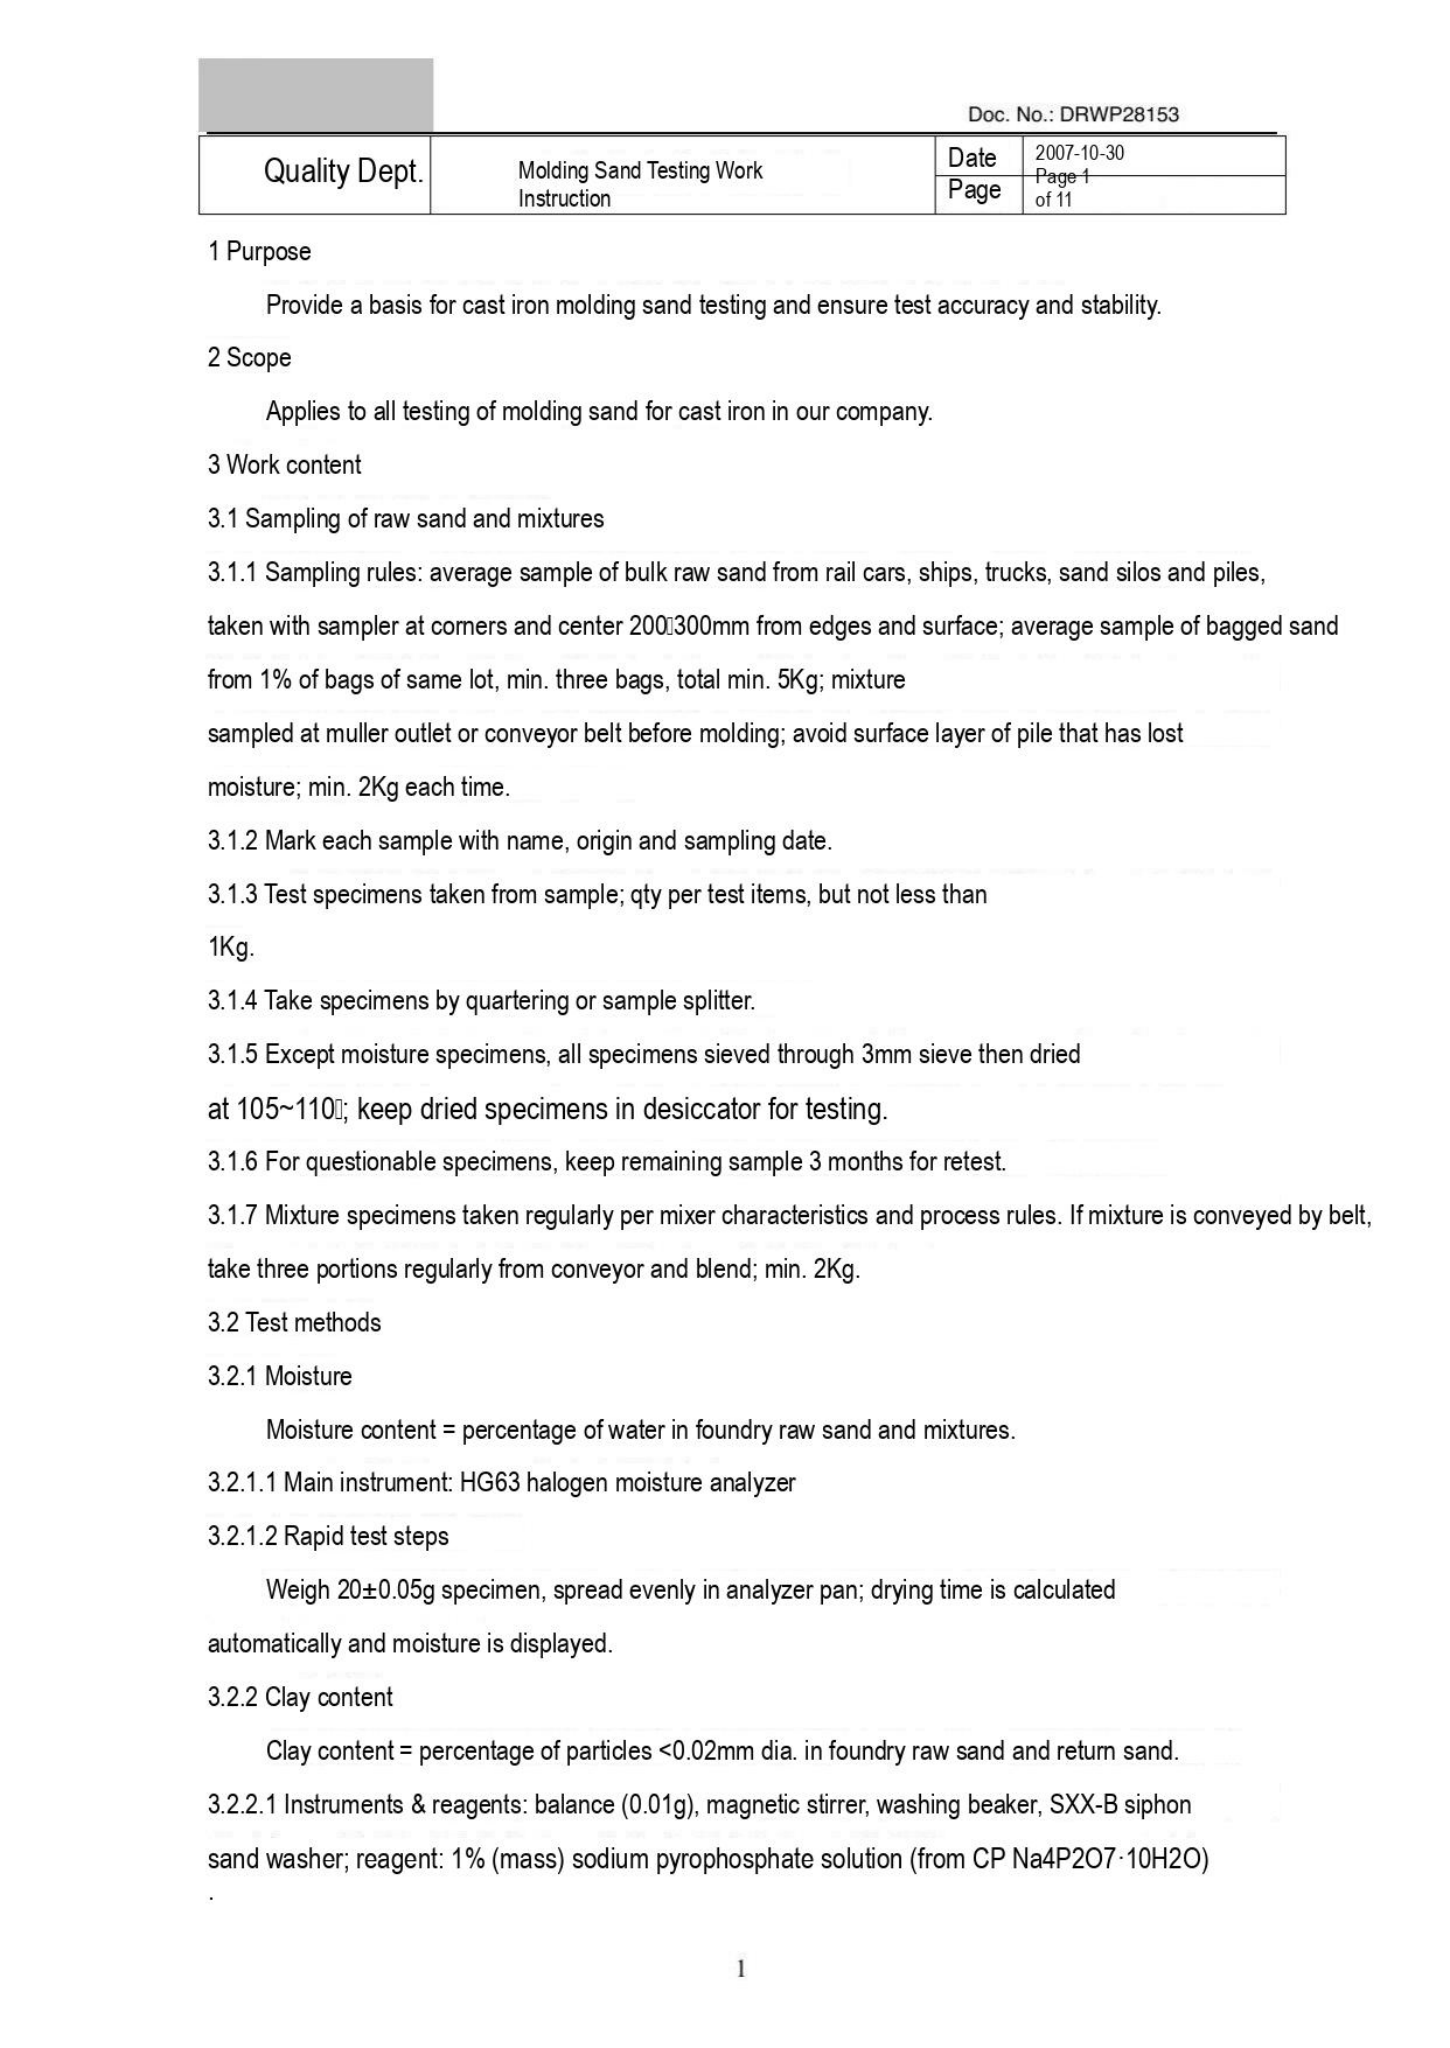Doc. No.: DRWP28153

| Quality Dept. | Molding Sand Testing Work Instruction | Date | 2007-10-30 |
|---|---|---|---|
| | | Page | Page 1 of 11 |

1 Purpose

Provide a basis for cast iron molding sand testing and ensure test accuracy and stability.

2 Scope

Applies to all testing of molding sand for cast iron in our company.

3 Work content

3.1 Sampling of raw sand and mixtures

3.1.1 Sampling rules: average sample of bulk raw sand from rail cars, ships, trucks, sand silos and piles, taken with sampler at corners and center 200300mm from edges and surface; average sample of bagged sand from 1% of bags of same lot, min. three bags, total min. 5Kg; mixture sampled at muller outlet or conveyor belt before molding; avoid surface layer of pile that has lost moisture; min. 2Kg each time.

3.1.2 Mark each sample with name, origin and sampling date.

3.1.3 Test specimens taken from sample; qty per test items, but not less than 1Kg.

3.1.4 Take specimens by quartering or sample splitter.

3.1.5 Except moisture specimens, all specimens sieved through 3mm sieve then dried at 105~110; keep dried specimens in desiccator for testing.

3.1.6 For questionable specimens, keep remaining sample 3 months for retest.

3.1.7 Mixture specimens taken regularly per mixer characteristics and process rules. If mixture is conveyed by belt, take three portions regularly from conveyor and blend; min. 2Kg.

3.2 Test methods

3.2.1 Moisture

Moisture content = percentage of water in foundry raw sand and mixtures.

3.2.1.1 Main instrument: HG63 halogen moisture analyzer

3.2.1.2 Rapid test steps

Weigh 20±0.05g specimen, spread evenly in analyzer pan; drying time is calculated automatically and moisture is displayed.

3.2.2 Clay content

Clay content = percentage of particles <0.02mm dia. in foundry raw sand and return sand.

3.2.2.1 Instruments & reagents: balance (0.01g), magnetic stirrer, washing beaker, SXX-B siphon sand washer; reagent: 1% (mass) sodium pyrophosphate solution (from CP Na4P2O7·10H2O)

.

1
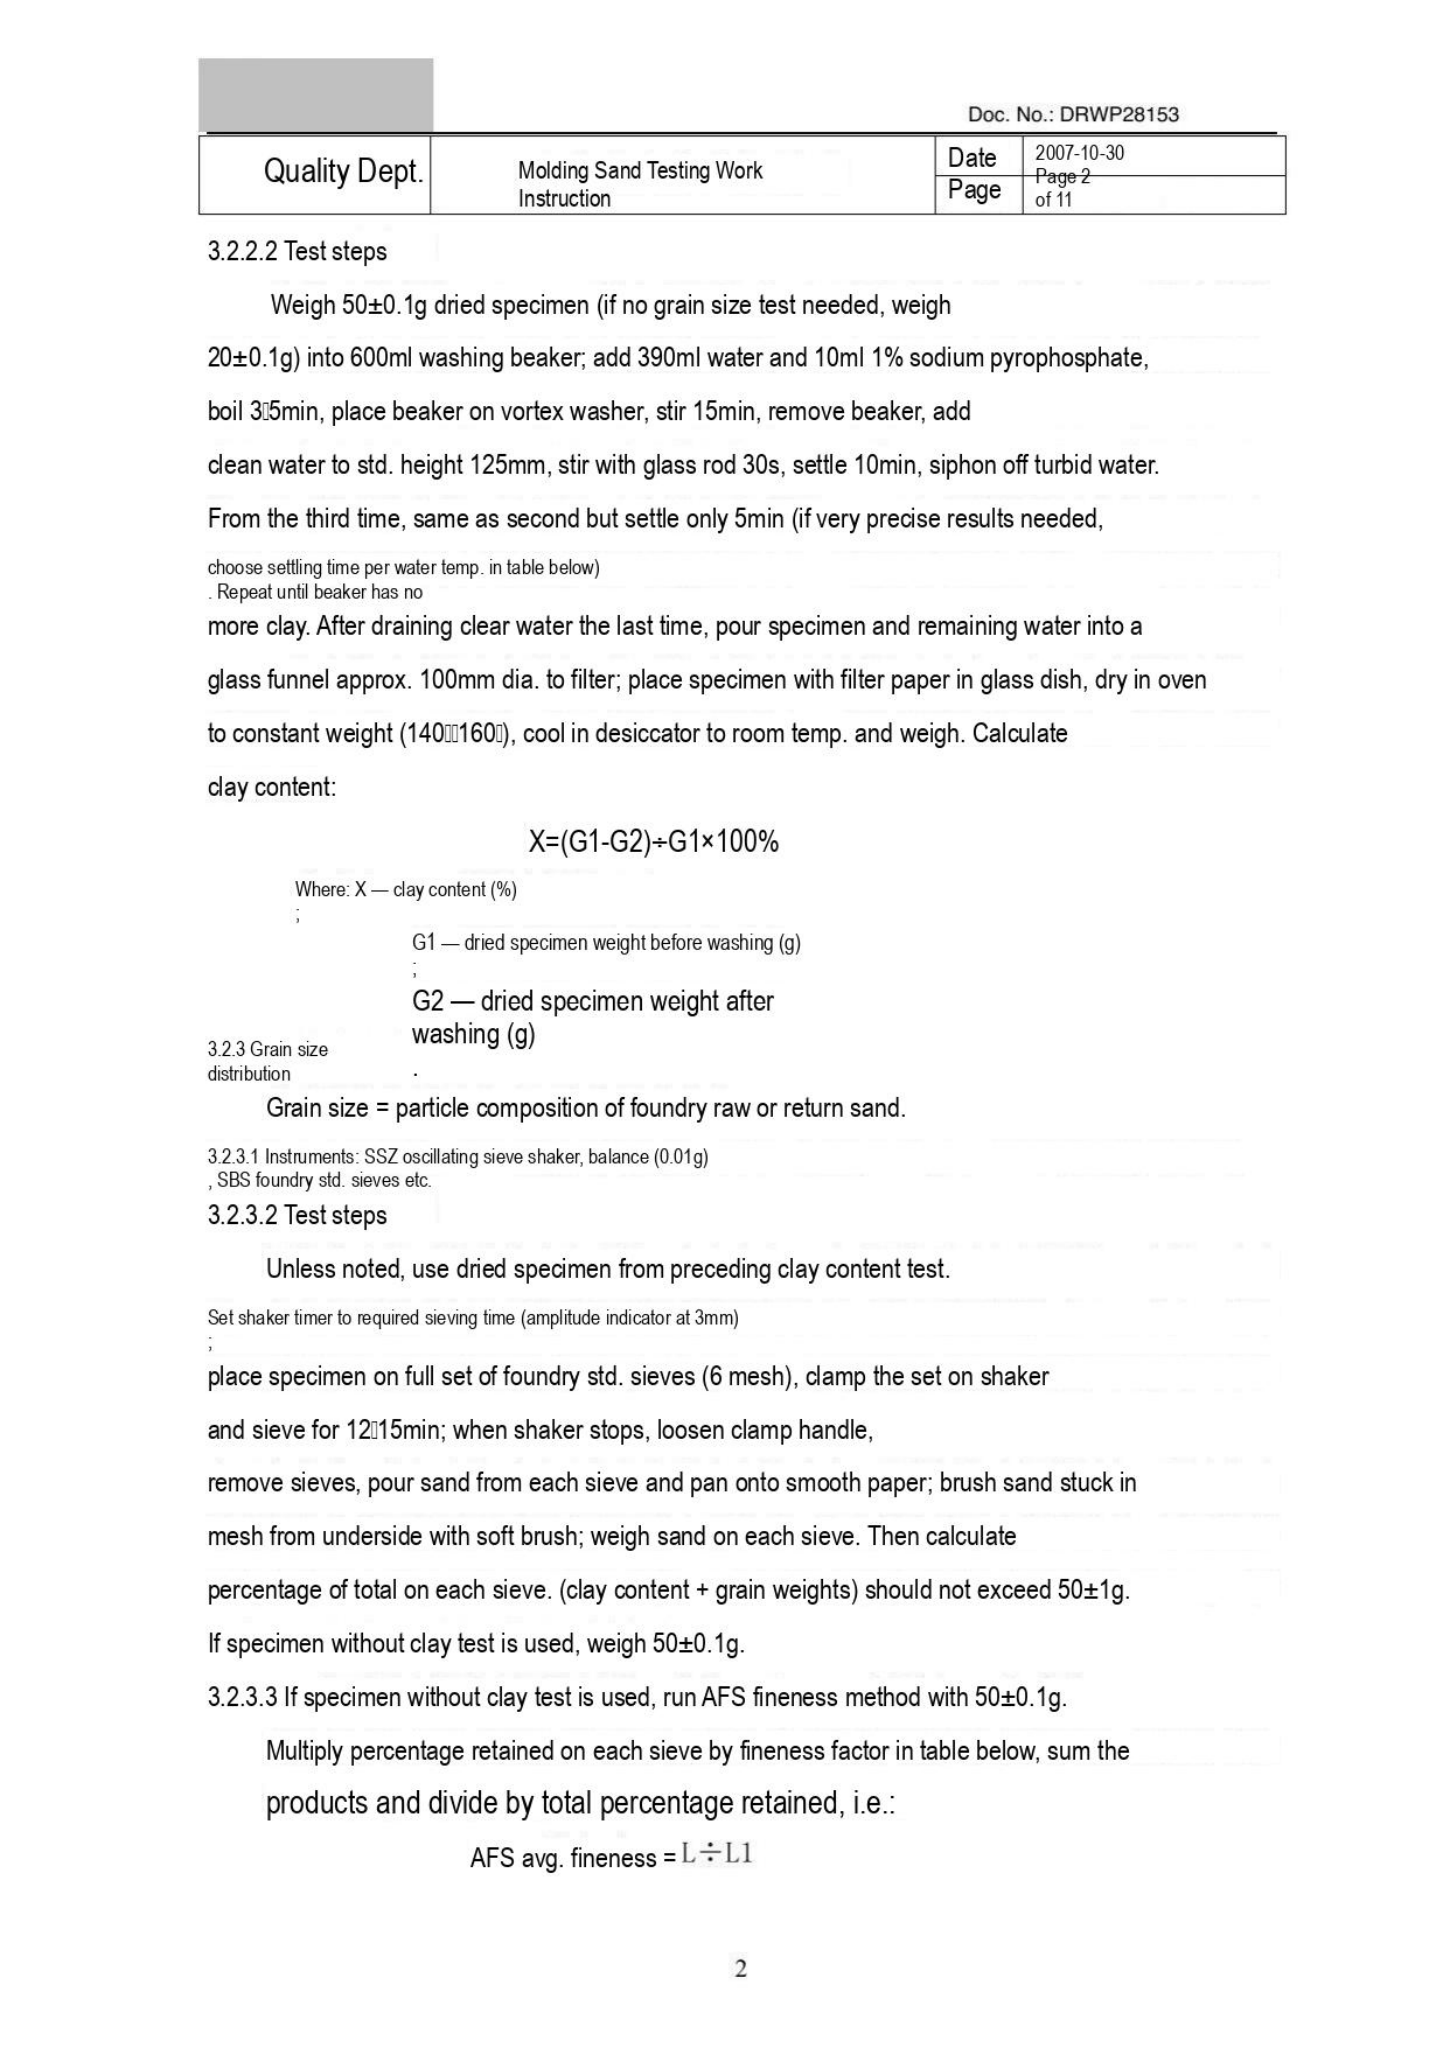Doc. No.: DRWP28153

| Quality Dept. | Molding Sand Testing Work Instruction | Date | 2007-10-30 |
|---|---|---|---|
| | | Page | Page 2 of 11 |

3.2.2.2 Test steps

Weigh 50±0.1g dried specimen (if no grain size test needed, weigh 20±0.1g) into 600ml washing beaker; add 390ml water and 10ml 1% sodium pyrophosphate, boil 35min, place beaker on vortex washer, stir 15min, remove beaker, add clean water to std. height 125mm, stir with glass rod 30s, settle 10min, siphon off turbid water. From the third time, same as second but settle only 5min (if very precise results needed, choose settling time per water temp. in table below). Repeat until beaker has no more clay. After draining clear water the last time, pour specimen and remaining water into a glass funnel approx. 100mm dia. to filter; place specimen with filter paper in glass dish, dry in oven to constant weight (140160), cool in desiccator to room temp. and weigh. Calculate clay content:

X=(G1-G2)÷G1×100%

Where: X — clay content (%);

G1 — dried specimen weight before washing (g);

G2 — dried specimen weight after washing (g).

3.2.3 Grain size distribution

Grain size = particle composition of foundry raw or return sand.

3.2.3.1 Instruments: SSZ oscillating sieve shaker, balance (0.01g), SBS foundry std. sieves etc.

3.2.3.2 Test steps

Unless noted, use dried specimen from preceding clay content test.

Set shaker timer to required sieving time (amplitude indicator at 3mm); place specimen on full set of foundry std. sieves (6 mesh), clamp the set on shaker and sieve for 1215min; when shaker stops, loosen clamp handle, remove sieves, pour sand from each sieve and pan onto smooth paper; brush sand stuck in mesh from underside with soft brush; weigh sand on each sieve. Then calculate percentage of total on each sieve. (clay content + grain weights) should not exceed 50±1g. If specimen without clay test is used, weigh 50±0.1g.

3.2.3.3 If specimen without clay test is used, run AFS fineness method with 50±0.1g.

Multiply percentage retained on each sieve by fineness factor in table below, sum the products and divide by total percentage retained, i.e.:

AFS avg. fineness = L÷L1

2
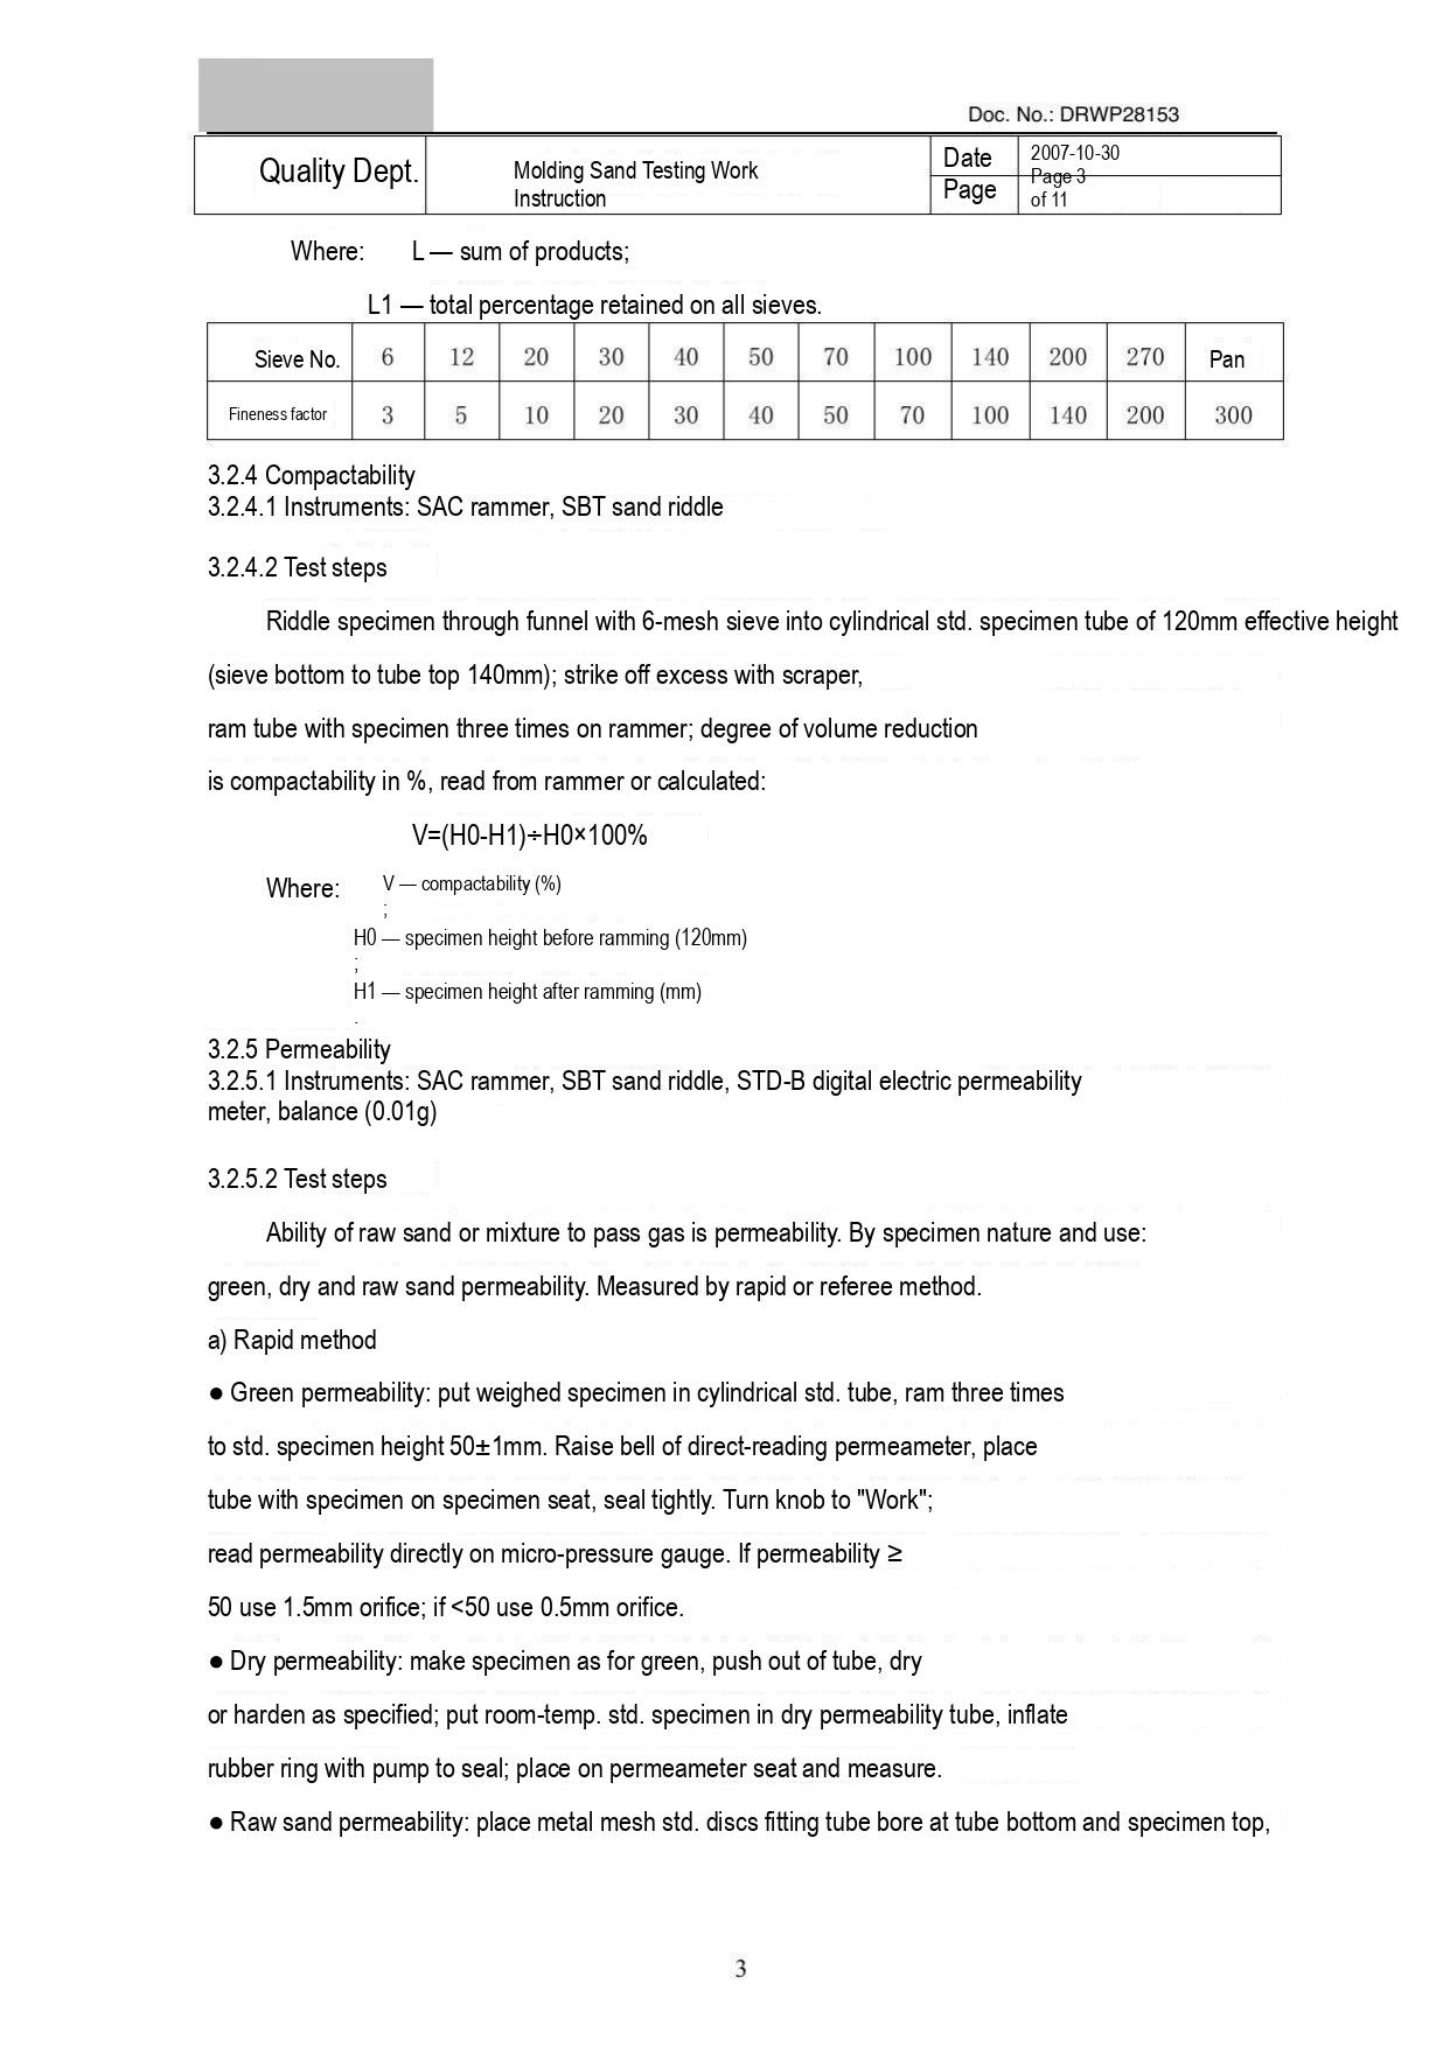Doc. No.: DRWP28153

| Quality Dept. | Molding Sand Testing Work Instruction | Date | 2007-10-30 |
|---|---|---|---|
| | | Page | Page 3 of 11 |

Where: L — sum of products;

L1 — total percentage retained on all sieves.

| Sieve No. | 6 | 12 | 20 | 30 | 40 | 50 | 70 | 100 | 140 | 200 | 270 | Pan |
|---|---|---|---|---|---|---|---|---|---|---|---|---|
| Fineness factor | 3 | 5 | 10 | 20 | 30 | 40 | 50 | 70 | 100 | 140 | 200 | 300 |

3.2.4 Compactability
3.2.4.1 Instruments: SAC rammer, SBT sand riddle

3.2.4.2 Test steps

Riddle specimen through funnel with 6-mesh sieve into cylindrical std. specimen tube of 120mm effective height (sieve bottom to tube top 140mm); strike off excess with scraper,

ram tube with specimen three times on rammer; degree of volume reduction

is compactability in %, read from rammer or calculated:

V=(H0-H1)÷H0×100%

Where: V — compactability (%)
;
H0 — specimen height before ramming (120mm)
;
H1 — specimen height after ramming (mm)
.

3.2.5 Permeability
3.2.5.1 Instruments: SAC rammer, SBT sand riddle, STD-B digital electric permeability meter, balance (0.01g)

3.2.5.2 Test steps

Ability of raw sand or mixture to pass gas is permeability. By specimen nature and use:

green, dry and raw sand permeability. Measured by rapid or referee method.

a) Rapid method

● Green permeability: put weighed specimen in cylindrical std. tube, ram three times

to std. specimen height 50±1mm. Raise bell of direct-reading permeameter, place

tube with specimen on specimen seat, seal tightly. Turn knob to "Work";

read permeability directly on micro-pressure gauge. If permeability ≥

50 use 1.5mm orifice; if <50 use 0.5mm orifice.

● Dry permeability: make specimen as for green, push out of tube, dry

or harden as specified; put room-temp. std. specimen in dry permeability tube, inflate

rubber ring with pump to seal; place on permeameter seat and measure.

● Raw sand permeability: place metal mesh std. discs fitting tube bore at tube bottom and specimen top,

3
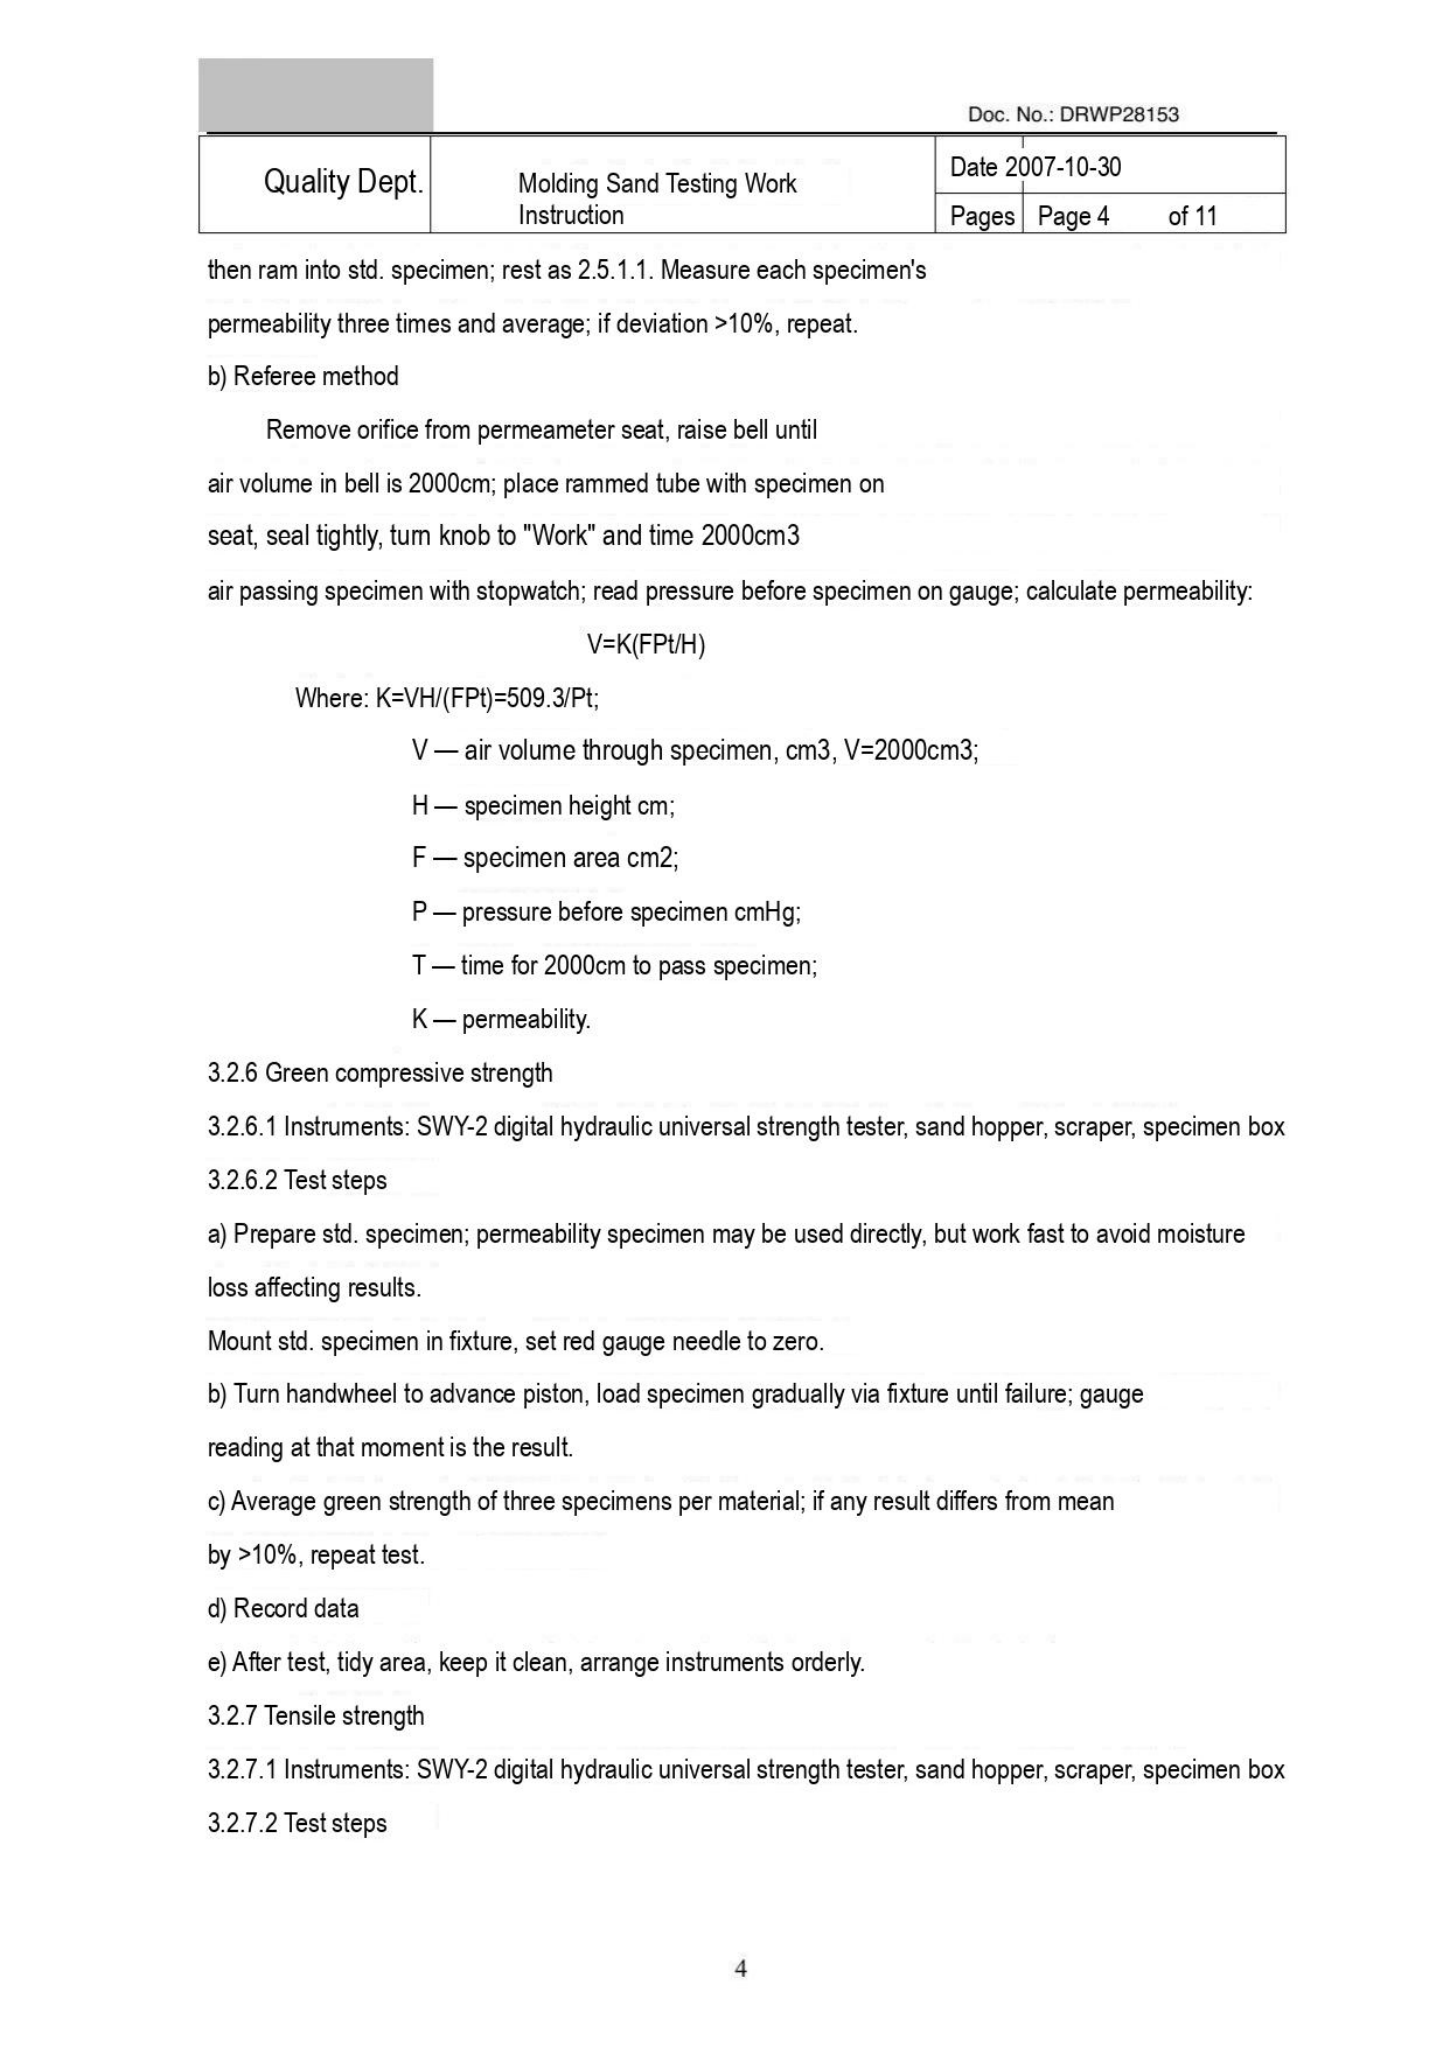Doc. No.: DRWP28153

| Quality Dept. | Molding Sand Testing Work Instruction | Date 2007-10-30 | |
|---|---|---|---|
| | | Pages | Page 4 of 11 |

then ram into std. specimen; rest as 2.5.1.1. Measure each specimen's

permeability three times and average; if deviation >10%, repeat.

b) Referee method

Remove orifice from permeameter seat, raise bell until

air volume in bell is 2000cm; place rammed tube with specimen on

seat, seal tightly, turn knob to "Work" and time 2000cm3

air passing specimen with stopwatch; read pressure before specimen on gauge; calculate permeability:

V=K(FPt/H)

Where: K=VH/(FPt)=509.3/Pt;

V — air volume through specimen, cm3, V=2000cm3;

H — specimen height cm;

F — specimen area cm2;

P — pressure before specimen cmHg;

T — time for 2000cm to pass specimen;

K — permeability.

3.2.6 Green compressive strength

3.2.6.1 Instruments: SWY-2 digital hydraulic universal strength tester, sand hopper, scraper, specimen box

3.2.6.2 Test steps

a) Prepare std. specimen; permeability specimen may be used directly, but work fast to avoid moisture loss affecting results.

Mount std. specimen in fixture, set red gauge needle to zero.

b) Turn handwheel to advance piston, load specimen gradually via fixture until failure; gauge reading at that moment is the result.

c) Average green strength of three specimens per material; if any result differs from mean by >10%, repeat test.

d) Record data

e) After test, tidy area, keep it clean, arrange instruments orderly.

3.2.7 Tensile strength

3.2.7.1 Instruments: SWY-2 digital hydraulic universal strength tester, sand hopper, scraper, specimen box

3.2.7.2 Test steps

4
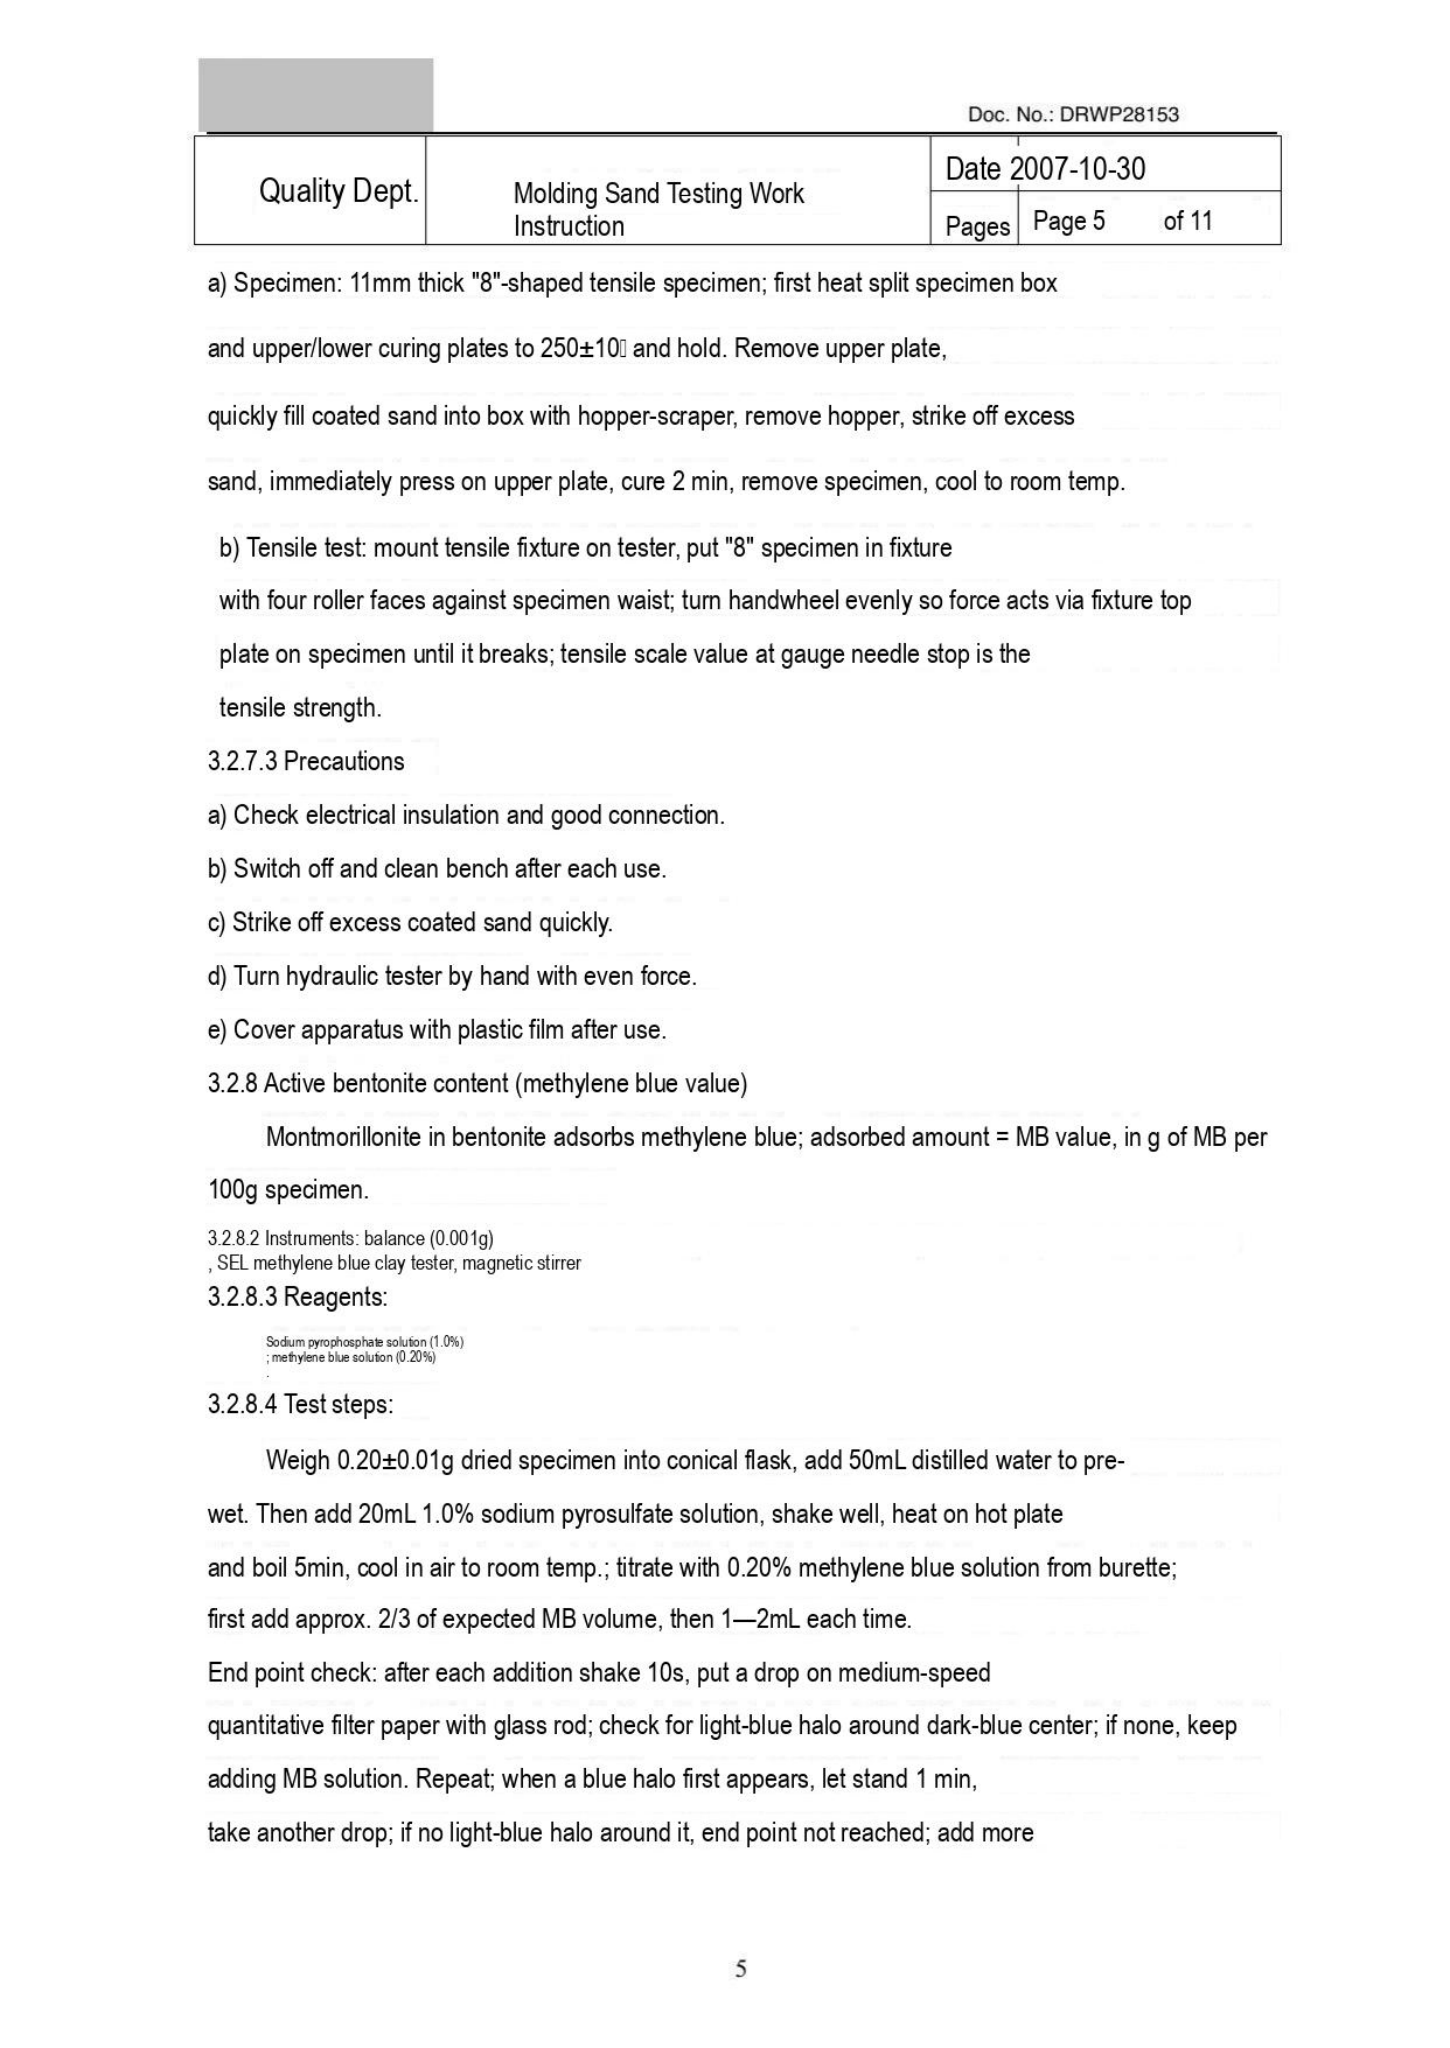Doc. No.: DRWP28153

| Quality Dept. | Molding Sand Testing Work Instruction | Date 2007-10-30 | |
|---|---|---|---|
| | | Pages | Page 5 of 11 |

a) Specimen: 11mm thick "8"-shaped tensile specimen; first heat split specimen box

and upper/lower curing plates to 250±10 and hold. Remove upper plate,

quickly fill coated sand into box with hopper-scraper, remove hopper, strike off excess

sand, immediately press on upper plate, cure 2 min, remove specimen, cool to room temp.

b) Tensile test: mount tensile fixture on tester, put "8" specimen in fixture

with four roller faces against specimen waist; turn handwheel evenly so force acts via fixture top

plate on specimen until it breaks; tensile scale value at gauge needle stop is the

tensile strength.

3.2.7.3 Precautions

a) Check electrical insulation and good connection.

b) Switch off and clean bench after each use.

c) Strike off excess coated sand quickly.

d) Turn hydraulic tester by hand with even force.

e) Cover apparatus with plastic film after use.

3.2.8 Active bentonite content (methylene blue value)

Montmorillonite in bentonite adsorbs methylene blue; adsorbed amount = MB value, in g of MB per 100g specimen.

3.2.8.2 Instruments: balance (0.001g)
, SEL methylene blue clay tester, magnetic stirrer

3.2.8.3 Reagents:

Sodium pyrophosphate solution (1.0%)
; methylene blue solution (0.20%)

3.2.8.4 Test steps:

Weigh 0.20±0.01g dried specimen into conical flask, add 50mL distilled water to pre-wet. Then add 20mL 1.0% sodium pyrosulfate solution, shake well, heat on hot plate

and boil 5min, cool in air to room temp.; titrate with 0.20% methylene blue solution from burette;

first add approx. 2/3 of expected MB volume, then 1—2mL each time.

End point check: after each addition shake 10s, put a drop on medium-speed

quantitative filter paper with glass rod; check for light-blue halo around dark-blue center; if none, keep

adding MB solution. Repeat; when a blue halo first appears, let stand 1 min,

take another drop; if no light-blue halo around it, end point not reached; add more

5
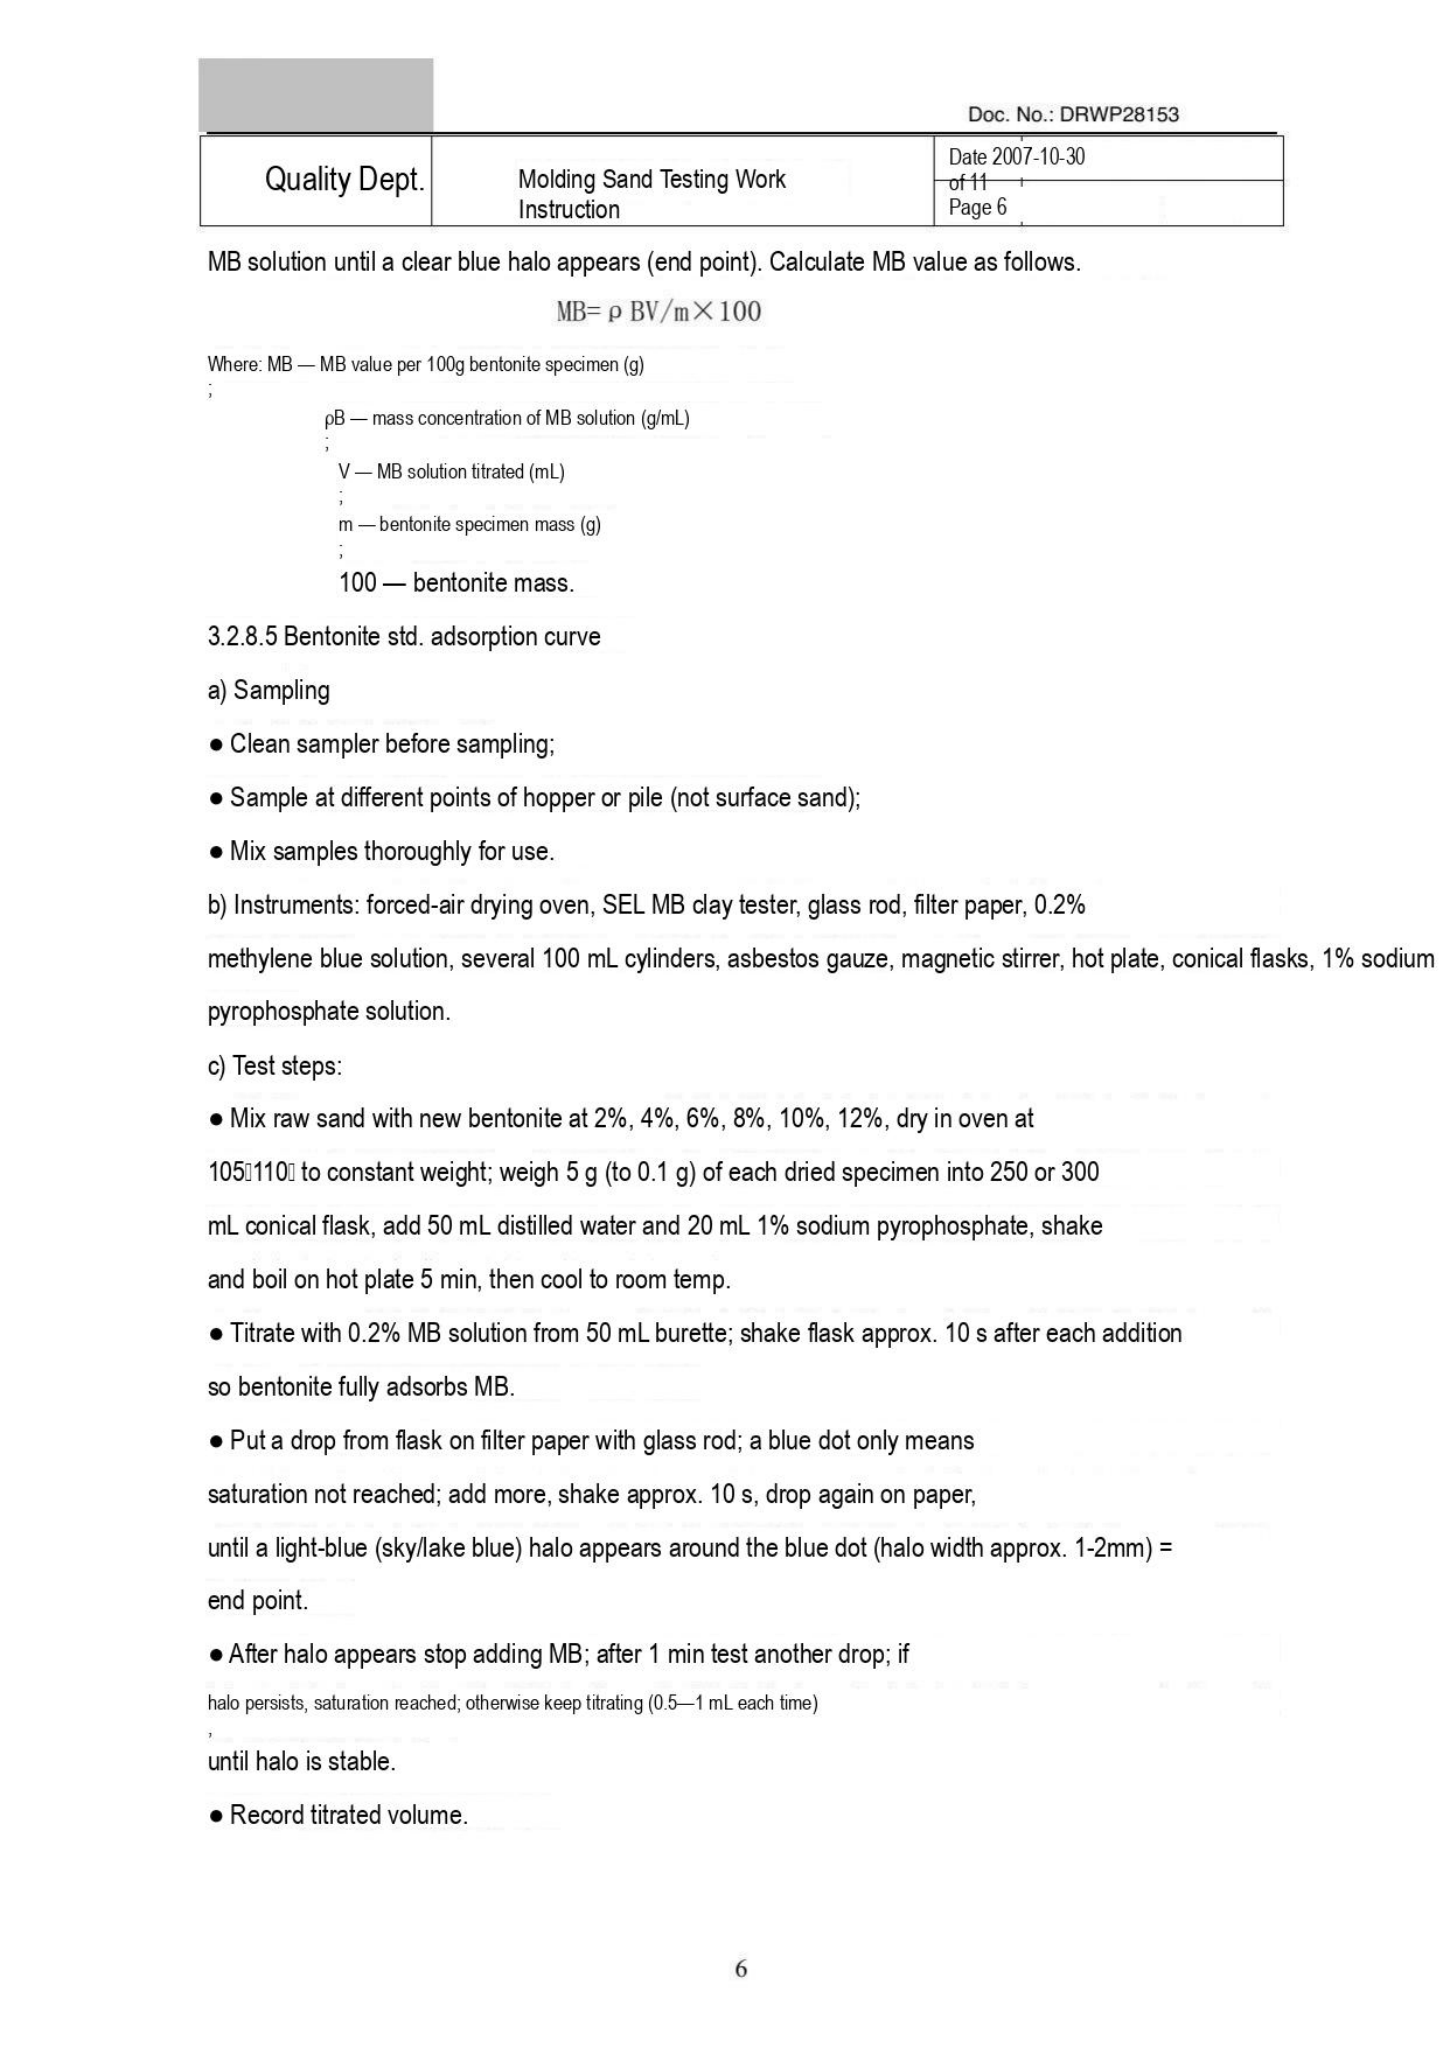Doc. No.: DRWP28153

| Quality Dept. | Molding Sand Testing Work Instruction | Date 2007-10-30<br>of 11<br>Page 6 |
|---|---|---|

MB solution until a clear blue halo appears (end point). Calculate MB value as follows.

MB= ρ BV/m×100

Where: MB — MB value per 100g bentonite specimen (g)
;
ρB — mass concentration of MB solution (g/mL)
;
V — MB solution titrated (mL)
;
m — bentonite specimen mass (g)
;
100 — bentonite mass.

3.2.8.5 Bentonite std. adsorption curve

a) Sampling

● Clean sampler before sampling;

● Sample at different points of hopper or pile (not surface sand);

● Mix samples thoroughly for use.

b) Instruments: forced-air drying oven, SEL MB clay tester, glass rod, filter paper, 0.2%

methylene blue solution, several 100 mL cylinders, asbestos gauze, magnetic stirrer, hot plate, conical flasks, 1% sodium

pyrophosphate solution.

c) Test steps:

● Mix raw sand with new bentonite at 2%, 4%, 6%, 8%, 10%, 12%, dry in oven at

105110 to constant weight; weigh 5 g (to 0.1 g) of each dried specimen into 250 or 300

mL conical flask, add 50 mL distilled water and 20 mL 1% sodium pyrophosphate, shake

and boil on hot plate 5 min, then cool to room temp.

● Titrate with 0.2% MB solution from 50 mL burette; shake flask approx. 10 s after each addition

so bentonite fully adsorbs MB.

● Put a drop from flask on filter paper with glass rod; a blue dot only means

saturation not reached; add more, shake approx. 10 s, drop again on paper,

until a light-blue (sky/lake blue) halo appears around the blue dot (halo width approx. 1-2mm) =

end point.

● After halo appears stop adding MB; after 1 min test another drop; if

halo persists, saturation reached; otherwise keep titrating (0.5—1 mL each time)
,
until halo is stable.

● Record titrated volume.

6